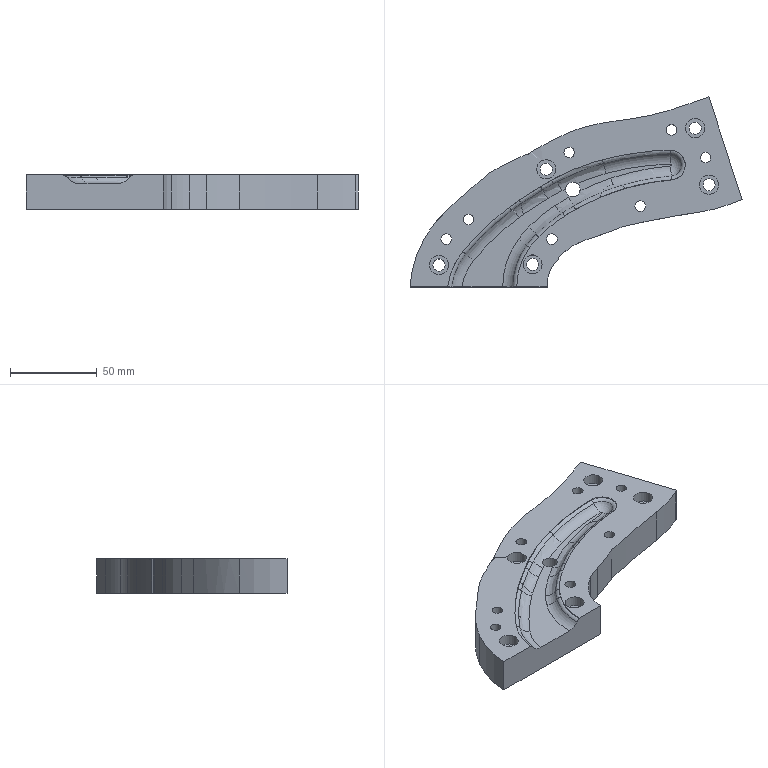Part | NX | features 23 2 | 1 solid | 98 faces | box 191.666 x 109.691 x 20 mm | volume 198445 mm3 | cylinder 35 | spline 29 | plane 20 | torus 14 | commonest cylinder face diameters 6.2 x5 7 x5 11 x5 4.4 x2 6.001 x2 8.5 x1